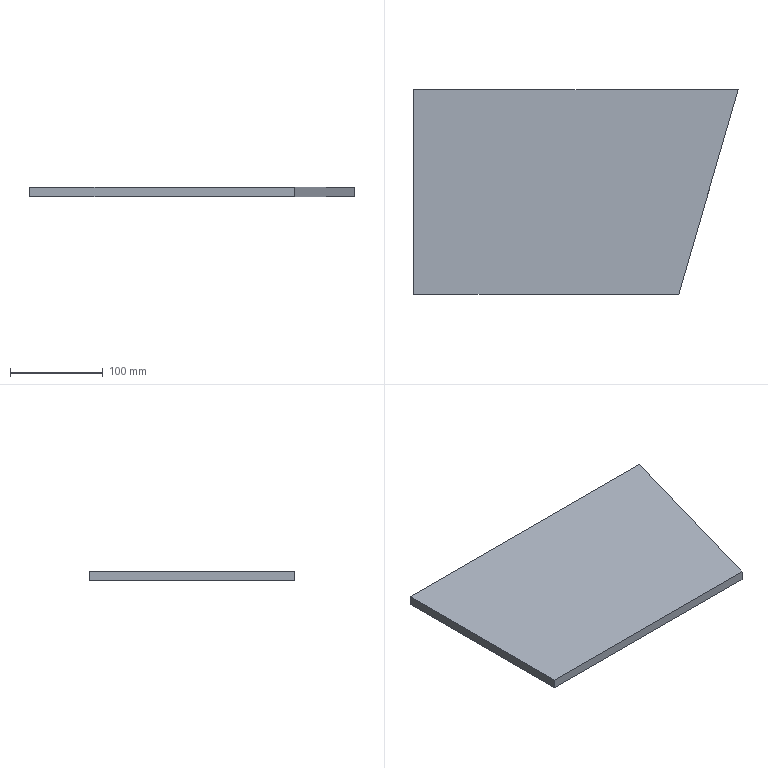Part | STEP file | 13-Steel plate | 1 solid | 6 faces | box 349 x 220 x 10 mm | volume 697400 mm3 | plane 6
STEP:
#1=CARTESIAN_POINT('',(0.,0.,0.));
#2=DIRECTION('',(0.,0.,1.));
#3=DIRECTION('',(1.,0.,0.));
#4=AXIS2_PLACEMENT_3D('',#1,#2,#3);
#5=CARTESIAN_POINT('',(0.,0.,0.));
#6=VERTEX_POINT('',#5);
#7=CARTESIAN_POINT('',(0.,-220.,0.));
#8=VERTEX_POINT('',#7);
#9=CARTESIAN_POINT('',(0.,0.,0.));
#10=DIRECTION('',(0.,-1.,0.));
#11=VECTOR('',#10,1.);
#12=LINE('',#9,#11);
#13=CARTESIAN_POINT('',(0.,0.,10.));
#14=DIRECTION('',(1.,0.,0.));
#15=DIRECTION('',(0.,1.,0.));
#16=AXIS2_PLACEMENT_3D('',#13,#14,#15);
#17=PLANE('',#16);
#18=CARTESIAN_POINT('',(0.,-10.));
#19=DIRECTION('',(-1.,0.));
#20=VECTOR('',#19,1.);
#21=LINE('',#18,#20);
#22=(GEOMETRIC_REPRESENTATION_CONTEXT(2)PARAMETRIC_REPRESENTATION_CONTEXT()REPRESENTATION_CONTEXT('',''));
#23=DEFINITIONAL_REPRESENTATION('',(#21),#22);
#24=PCURVE('',#17,#23);
#25=CARTESIAN_POINT('',(0.,0.,0.));
#26=DIRECTION('',(0.,0.,1.));
#27=DIRECTION('',(1.,0.,0.));
#28=AXIS2_PLACEMENT_3D('',#25,#26,#27);
#29=PLANE('',#28);
#30=CARTESIAN_POINT('',(0.,0.));
#31=DIRECTION('',(0.,-1.));
#32=VECTOR('',#31,1.);
#33=LINE('',#30,#32);
#34=(GEOMETRIC_REPRESENTATION_CONTEXT(2)PARAMETRIC_REPRESENTATION_CONTEXT()REPRESENTATION_CONTEXT('',''));
#35=DEFINITIONAL_REPRESENTATION('',(#33),#34);
#36=PCURVE('',#29,#35);
#37=SURFACE_CURVE('',#12,(#24,#36),.PCURVE_S1.);
#38=EDGE_CURVE('',#6,#8,#37,.T.);
#39=ORIENTED_EDGE('',*,*,#38,.T.);
#40=CARTESIAN_POINT('',(0.,-220.,10.));
#41=VERTEX_POINT('',#40);
#42=CARTESIAN_POINT('',(0.,-220.,10.));
#43=DIRECTION('',(0.,0.,-1.));
#44=VECTOR('',#43,1.);
#45=LINE('',#42,#44);
#46=CARTESIAN_POINT('',(-220.,0.));
#47=DIRECTION('',(0.,-1.));
#48=VECTOR('',#47,1.);
#49=LINE('',#46,#48);
#50=(GEOMETRIC_REPRESENTATION_CONTEXT(2)PARAMETRIC_REPRESENTATION_CONTEXT()REPRESENTATION_CONTEXT('',''));
#51=DEFINITIONAL_REPRESENTATION('',(#49),#50);
#52=PCURVE('',#17,#51);
#53=CARTESIAN_POINT('',(0.,-220.,10.));
#54=DIRECTION('',(0.,1.,0.));
#55=DIRECTION('',(0.,0.,1.));
#56=AXIS2_PLACEMENT_3D('',#53,#54,#55);
#57=PLANE('',#56);
#58=CARTESIAN_POINT('',(0.,0.));
#59=DIRECTION('',(-1.,0.));
#60=VECTOR('',#59,1.);
#61=LINE('',#58,#60);
#62=(GEOMETRIC_REPRESENTATION_CONTEXT(2)PARAMETRIC_REPRESENTATION_CONTEXT()REPRESENTATION_CONTEXT('',''));
#63=DEFINITIONAL_REPRESENTATION('',(#61),#62);
#64=PCURVE('',#57,#63);
#65=SURFACE_CURVE('',#45,(#52,#64),.PCURVE_S1.);
#66=EDGE_CURVE('',#41,#8,#65,.T.);
#67=ORIENTED_EDGE('',*,*,#66,.F.);
#68=CARTESIAN_POINT('',(0.,0.,10.));
#69=VERTEX_POINT('',#68);
#70=CARTESIAN_POINT('',(0.,0.,10.));
#71=DIRECTION('',(0.,-1.,0.));
#72=VECTOR('',#71,1.);
#73=LINE('',#70,#72);
#74=CARTESIAN_POINT('',(0.,0.));
#75=DIRECTION('',(-1.,0.));
#76=VECTOR('',#75,1.);
#77=LINE('',#74,#76);
#78=(GEOMETRIC_REPRESENTATION_CONTEXT(2)PARAMETRIC_REPRESENTATION_CONTEXT()REPRESENTATION_CONTEXT('',''));
#79=DEFINITIONAL_REPRESENTATION('',(#77),#78);
#80=PCURVE('',#17,#79);
#81=CARTESIAN_POINT('',(0.,0.,10.));
#82=DIRECTION('',(0.,0.,1.));
#83=DIRECTION('',(1.,0.,0.));
#84=AXIS2_PLACEMENT_3D('',#81,#82,#83);
#85=PLANE('',#84);
#86=CARTESIAN_POINT('',(0.,0.));
#87=DIRECTION('',(0.,-1.));
#88=VECTOR('',#87,1.);
#89=LINE('',#86,#88);
#90=(GEOMETRIC_REPRESENTATION_CONTEXT(2)PARAMETRIC_REPRESENTATION_CONTEXT()REPRESENTATION_CONTEXT('',''));
#91=DEFINITIONAL_REPRESENTATION('',(#89),#90);
#92=PCURVE('',#85,#91);
#93=SURFACE_CURVE('',#73,(#80,#92),.PCURVE_S1.);
#94=EDGE_CURVE('',#69,#41,#93,.T.);
#95=ORIENTED_EDGE('',*,*,#94,.F.);
#96=CARTESIAN_POINT('',(0.,0.,10.));
#97=DIRECTION('',(0.,0.,-1.));
#98=VECTOR('',#97,1.);
#99=LINE('',#96,#98);
#100=CARTESIAN_POINT('',(0.,0.));
#101=DIRECTION('',(0.,-1.));
#102=VECTOR('',#101,1.);
#103=LINE('',#100,#102);
#104=(GEOMETRIC_REPRESENTATION_CONTEXT(2)PARAMETRIC_REPRESENTATION_CONTEXT()REPRESENTATION_CONTEXT('',''));
#105=DEFINITIONAL_REPRESENTATION('',(#103),#104);
#106=PCURVE('',#17,#105);
#107=CARTESIAN_POINT('',(0.,0.,10.));
#108=DIRECTION('',(0.,-1.,0.));
#109=DIRECTION('',(0.,0.,-1.));
#110=AXIS2_PLACEMENT_3D('',#107,#108,#109);
#111=PLANE('',#110);
#112=CARTESIAN_POINT('',(0.,0.));
#113=DIRECTION('',(1.,0.));
#114=VECTOR('',#113,1.);
#115=LINE('',#112,#114);
#116=(GEOMETRIC_REPRESENTATION_CONTEXT(2)PARAMETRIC_REPRESENTATION_CONTEXT()REPRESENTATION_CONTEXT('',''));
#117=DEFINITIONAL_REPRESENTATION('',(#115),#116);
#118=PCURVE('',#111,#117);
#119=SURFACE_CURVE('',#99,(#106,#118),.PCURVE_S1.);
#120=EDGE_CURVE('',#69,#6,#119,.T.);
#121=ORIENTED_EDGE('',*,*,#120,.T.);
#122=EDGE_LOOP('',(#39,#67,#95,#121));
#123=FACE_BOUND('',#122,.T.);
#124=ADVANCED_FACE('',(#123),#17,.F.);
#125=CARTESIAN_POINT('',(285.,-220.,0.));
#126=VERTEX_POINT('',#125);
#127=CARTESIAN_POINT('',(0.,-220.,0.));
#128=DIRECTION('',(1.,0.,0.));
#129=VECTOR('',#128,1.);
#130=LINE('',#127,#129);
#131=CARTESIAN_POINT('',(-10.,0.));
#132=DIRECTION('',(0.,1.));
#133=VECTOR('',#132,1.);
#134=LINE('',#131,#133);
#135=(GEOMETRIC_REPRESENTATION_CONTEXT(2)PARAMETRIC_REPRESENTATION_CONTEXT()REPRESENTATION_CONTEXT('',''));
#136=DEFINITIONAL_REPRESENTATION('',(#134),#135);
#137=PCURVE('',#57,#136);
#138=CARTESIAN_POINT('',(0.,-220.));
#139=DIRECTION('',(1.,0.));
#140=VECTOR('',#139,1.);
#141=LINE('',#138,#140);
#142=(GEOMETRIC_REPRESENTATION_CONTEXT(2)PARAMETRIC_REPRESENTATION_CONTEXT()REPRESENTATION_CONTEXT('',''));
#143=DEFINITIONAL_REPRESENTATION('',(#141),#142);
#144=PCURVE('',#29,#143);
#145=SURFACE_CURVE('',#130,(#137,#144),.PCURVE_S1.);
#146=EDGE_CURVE('',#8,#126,#145,.T.);
#147=ORIENTED_EDGE('',*,*,#146,.T.);
#148=CARTESIAN_POINT('',(285.,-220.,10.));
#149=VERTEX_POINT('',#148);
#150=CARTESIAN_POINT('',(285.,-220.,10.));
#151=DIRECTION('',(0.,0.,-1.));
#152=VECTOR('',#151,1.);
#153=LINE('',#150,#152);
#154=CARTESIAN_POINT('',(0.,285.));
#155=DIRECTION('',(-1.,0.));
#156=VECTOR('',#155,1.);
#157=LINE('',#154,#156);
#158=(GEOMETRIC_REPRESENTATION_CONTEXT(2)PARAMETRIC_REPRESENTATION_CONTEXT()REPRESENTATION_CONTEXT('',''));
#159=DEFINITIONAL_REPRESENTATION('',(#157),#158);
#160=PCURVE('',#57,#159);
#161=CARTESIAN_POINT('',(349.,0.,10.));
#162=DIRECTION('',(-0.9602,0.2793,0.));
#163=DIRECTION('',(-0.2793,-0.9602,0.));
#164=AXIS2_PLACEMENT_3D('',#161,#162,#163);
#165=PLANE('',#164);
#166=CARTESIAN_POINT('',(229.12,0.));
#167=DIRECTION('',(0.,-1.));
#168=VECTOR('',#167,1.);
#169=LINE('',#166,#168);
#170=(GEOMETRIC_REPRESENTATION_CONTEXT(2)PARAMETRIC_REPRESENTATION_CONTEXT()REPRESENTATION_CONTEXT('',''));
#171=DEFINITIONAL_REPRESENTATION('',(#169),#170);
#172=PCURVE('',#165,#171);
#173=SURFACE_CURVE('',#153,(#160,#172),.PCURVE_S1.);
#174=EDGE_CURVE('',#149,#126,#173,.T.);
#175=ORIENTED_EDGE('',*,*,#174,.F.);
#176=CARTESIAN_POINT('',(0.,-220.,10.));
#177=DIRECTION('',(1.,0.,0.));
#178=VECTOR('',#177,1.);
#179=LINE('',#176,#178);
#180=CARTESIAN_POINT('',(0.,0.));
#181=DIRECTION('',(0.,1.));
#182=VECTOR('',#181,1.);
#183=LINE('',#180,#182);
#184=(GEOMETRIC_REPRESENTATION_CONTEXT(2)PARAMETRIC_REPRESENTATION_CONTEXT()REPRESENTATION_CONTEXT('',''));
#185=DEFINITIONAL_REPRESENTATION('',(#183),#184);
#186=PCURVE('',#57,#185);
#187=CARTESIAN_POINT('',(0.,-220.));
#188=DIRECTION('',(1.,0.));
#189=VECTOR('',#188,1.);
#190=LINE('',#187,#189);
#191=(GEOMETRIC_REPRESENTATION_CONTEXT(2)PARAMETRIC_REPRESENTATION_CONTEXT()REPRESENTATION_CONTEXT('',''));
#192=DEFINITIONAL_REPRESENTATION('',(#190),#191);
#193=PCURVE('',#85,#192);
#194=SURFACE_CURVE('',#179,(#186,#193),.PCURVE_S1.);
#195=EDGE_CURVE('',#41,#149,#194,.T.);
#196=ORIENTED_EDGE('',*,*,#195,.F.);
#197=ORIENTED_EDGE('',*,*,#66,.T.);
#198=EDGE_LOOP('',(#147,#175,#196,#197));
#199=FACE_BOUND('',#198,.T.);
#200=ADVANCED_FACE('',(#199),#57,.F.);
#201=CARTESIAN_POINT('',(349.,0.,0.));
#202=VERTEX_POINT('',#201);
#203=CARTESIAN_POINT('',(349.,0.,0.));
#204=DIRECTION('',(0.2793,0.9602,0.));
#205=VECTOR('',#204,1.);
#206=LINE('',#203,#205);
#207=CARTESIAN_POINT('',(0.,-10.));
#208=DIRECTION('',(-1.,0.));
#209=VECTOR('',#208,1.);
#210=LINE('',#207,#209);
#211=(GEOMETRIC_REPRESENTATION_CONTEXT(2)PARAMETRIC_REPRESENTATION_CONTEXT()REPRESENTATION_CONTEXT('',''));
#212=DEFINITIONAL_REPRESENTATION('',(#210),#211);
#213=PCURVE('',#165,#212);
#214=CARTESIAN_POINT('',(349.,0.));
#215=DIRECTION('',(0.2793,0.9602));
#216=VECTOR('',#215,1.);
#217=LINE('',#214,#216);
#218=(GEOMETRIC_REPRESENTATION_CONTEXT(2)PARAMETRIC_REPRESENTATION_CONTEXT()REPRESENTATION_CONTEXT('',''));
#219=DEFINITIONAL_REPRESENTATION('',(#217),#218);
#220=PCURVE('',#29,#219);
#221=SURFACE_CURVE('',#206,(#213,#220),.PCURVE_S1.);
#222=EDGE_CURVE('',#126,#202,#221,.T.);
#223=ORIENTED_EDGE('',*,*,#222,.T.);
#224=CARTESIAN_POINT('',(349.,0.,10.));
#225=VERTEX_POINT('',#224);
#226=CARTESIAN_POINT('',(349.,0.,10.));
#227=DIRECTION('',(0.,0.,-1.));
#228=VECTOR('',#227,1.);
#229=LINE('',#226,#228);
#230=CARTESIAN_POINT('',(0.,0.));
#231=DIRECTION('',(0.,-1.));
#232=VECTOR('',#231,1.);
#233=LINE('',#230,#232);
#234=(GEOMETRIC_REPRESENTATION_CONTEXT(2)PARAMETRIC_REPRESENTATION_CONTEXT()REPRESENTATION_CONTEXT('',''));
#235=DEFINITIONAL_REPRESENTATION('',(#233),#234);
#236=PCURVE('',#165,#235);
#237=CARTESIAN_POINT('',(0.,349.));
#238=DIRECTION('',(1.,0.));
#239=VECTOR('',#238,1.);
#240=LINE('',#237,#239);
#241=(GEOMETRIC_REPRESENTATION_CONTEXT(2)PARAMETRIC_REPRESENTATION_CONTEXT()REPRESENTATION_CONTEXT('',''));
#242=DEFINITIONAL_REPRESENTATION('',(#240),#241);
#243=PCURVE('',#111,#242);
#244=SURFACE_CURVE('',#229,(#236,#243),.PCURVE_S1.);
#245=EDGE_CURVE('',#225,#202,#244,.T.);
#246=ORIENTED_EDGE('',*,*,#245,.F.);
#247=CARTESIAN_POINT('',(349.,0.,10.));
#248=DIRECTION('',(0.2793,0.9602,0.));
#249=VECTOR('',#248,1.);
#250=LINE('',#247,#249);
#251=CARTESIAN_POINT('',(0.,0.));
#252=DIRECTION('',(-1.,0.));
#253=VECTOR('',#252,1.);
#254=LINE('',#251,#253);
#255=(GEOMETRIC_REPRESENTATION_CONTEXT(2)PARAMETRIC_REPRESENTATION_CONTEXT()REPRESENTATION_CONTEXT('',''));
#256=DEFINITIONAL_REPRESENTATION('',(#254),#255);
#257=PCURVE('',#165,#256);
#258=CARTESIAN_POINT('',(349.,0.));
#259=DIRECTION('',(0.2793,0.9602));
#260=VECTOR('',#259,1.);
#261=LINE('',#258,#260);
#262=(GEOMETRIC_REPRESENTATION_CONTEXT(2)PARAMETRIC_REPRESENTATION_CONTEXT()REPRESENTATION_CONTEXT('',''));
#263=DEFINITIONAL_REPRESENTATION('',(#261),#262);
#264=PCURVE('',#85,#263);
#265=SURFACE_CURVE('',#250,(#257,#264),.PCURVE_S1.);
#266=EDGE_CURVE('',#149,#225,#265,.T.);
#267=ORIENTED_EDGE('',*,*,#266,.F.);
#268=ORIENTED_EDGE('',*,*,#174,.T.);
#269=EDGE_LOOP('',(#223,#246,#267,#268));
#270=FACE_BOUND('',#269,.T.);
#271=ADVANCED_FACE('',(#270),#165,.F.);
#272=CARTESIAN_POINT('',(0.,0.,0.));
#273=DIRECTION('',(-1.,0.,0.));
#274=VECTOR('',#273,1.);
#275=LINE('',#272,#274);
#276=CARTESIAN_POINT('',(10.,0.));
#277=DIRECTION('',(0.,-1.));
#278=VECTOR('',#277,1.);
#279=LINE('',#276,#278);
#280=(GEOMETRIC_REPRESENTATION_CONTEXT(2)PARAMETRIC_REPRESENTATION_CONTEXT()REPRESENTATION_CONTEXT('',''));
#281=DEFINITIONAL_REPRESENTATION('',(#279),#280);
#282=PCURVE('',#111,#281);
#283=CARTESIAN_POINT('',(0.,0.));
#284=DIRECTION('',(-1.,0.));
#285=VECTOR('',#284,1.);
#286=LINE('',#283,#285);
#287=(GEOMETRIC_REPRESENTATION_CONTEXT(2)PARAMETRIC_REPRESENTATION_CONTEXT()REPRESENTATION_CONTEXT('',''));
#288=DEFINITIONAL_REPRESENTATION('',(#286),#287);
#289=PCURVE('',#29,#288);
#290=SURFACE_CURVE('',#275,(#282,#289),.PCURVE_S1.);
#291=EDGE_CURVE('',#202,#6,#290,.T.);
#292=ORIENTED_EDGE('',*,*,#291,.T.);
#293=ORIENTED_EDGE('',*,*,#120,.F.);
#294=CARTESIAN_POINT('',(0.,0.,10.));
#295=DIRECTION('',(-1.,0.,0.));
#296=VECTOR('',#295,1.);
#297=LINE('',#294,#296);
#298=CARTESIAN_POINT('',(0.,0.));
#299=DIRECTION('',(0.,-1.));
#300=VECTOR('',#299,1.);
#301=LINE('',#298,#300);
#302=(GEOMETRIC_REPRESENTATION_CONTEXT(2)PARAMETRIC_REPRESENTATION_CONTEXT()REPRESENTATION_CONTEXT('',''));
#303=DEFINITIONAL_REPRESENTATION('',(#301),#302);
#304=PCURVE('',#111,#303);
#305=CARTESIAN_POINT('',(0.,0.));
#306=DIRECTION('',(-1.,0.));
#307=VECTOR('',#306,1.);
#308=LINE('',#305,#307);
#309=(GEOMETRIC_REPRESENTATION_CONTEXT(2)PARAMETRIC_REPRESENTATION_CONTEXT()REPRESENTATION_CONTEXT('',''));
#310=DEFINITIONAL_REPRESENTATION('',(#308),#309);
#311=PCURVE('',#85,#310);
#312=SURFACE_CURVE('',#297,(#304,#311),.PCURVE_S1.);
#313=EDGE_CURVE('',#225,#69,#312,.T.);
#314=ORIENTED_EDGE('',*,*,#313,.F.);
#315=ORIENTED_EDGE('',*,*,#245,.T.);
#316=EDGE_LOOP('',(#292,#293,#314,#315));
#317=FACE_BOUND('',#316,.T.);
#318=ADVANCED_FACE('',(#317),#111,.F.);
#319=ORIENTED_EDGE('',*,*,#94,.T.);
#320=ORIENTED_EDGE('',*,*,#195,.T.);
#321=ORIENTED_EDGE('',*,*,#266,.T.);
#322=ORIENTED_EDGE('',*,*,#313,.T.);
#323=EDGE_LOOP('',(#319,#320,#321,#322));
#324=FACE_BOUND('',#323,.T.);
#325=ADVANCED_FACE('',(#324),#85,.T.);
#326=ORIENTED_EDGE('',*,*,#38,.F.);
#327=ORIENTED_EDGE('',*,*,#291,.F.);
#328=ORIENTED_EDGE('',*,*,#222,.F.);
#329=ORIENTED_EDGE('',*,*,#146,.F.);
#330=EDGE_LOOP('',(#326,#327,#328,#329));
#331=FACE_BOUND('',#330,.T.);
#332=ADVANCED_FACE('',(#331),#29,.F.);
#333=CLOSED_SHELL('',(#124,#200,#271,#318,#325,#332));
#334=MANIFOLD_SOLID_BREP('',#333);
#335=(LENGTH_UNIT()NAMED_UNIT(*)SI_UNIT(.MILLI.,.METRE.));
#336=UNCERTAINTY_MEASURE_WITH_UNIT(LENGTH_MEASURE(0.0000001),#335,'','');
#337=(NAMED_UNIT(*)PLANE_ANGLE_UNIT()SI_UNIT($,.RADIAN.));
#338=(NAMED_UNIT(*)SI_UNIT($,.STERADIAN.)SOLID_ANGLE_UNIT());
#339=(GEOMETRIC_REPRESENTATION_CONTEXT(3)GLOBAL_UNCERTAINTY_ASSIGNED_CONTEXT((#336))GLOBAL_UNIT_ASSIGNED_CONTEXT((#335,#337,#338))REPRESENTATION_CONTEXT('',''));
#340=ADVANCED_BREP_SHAPE_REPRESENTATION('',(#4,#334),#339);